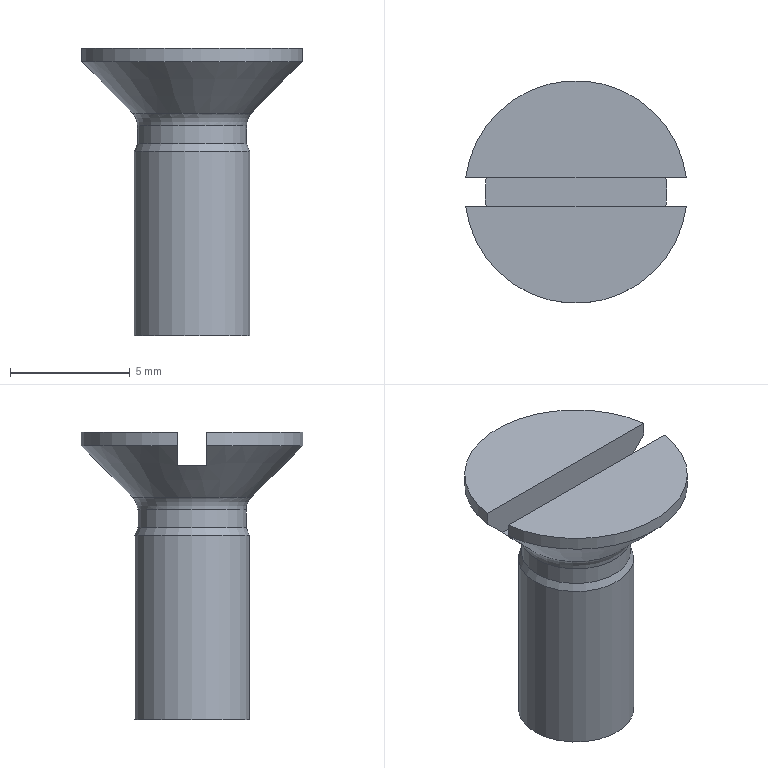Part | NX | features DATUM_CSYS 2, SKETCH 2, EXTRUDE 1, LINE 1, META 1, SWP104 1, SYMBOLIC_THREAD 1, THREADS 1 | 1 solid | 13 faces | box 9.222 x 9.3 x 12 mm | volume 279.35 mm3 | plane 6 | cylinder 4 | cone 2 | torus 1 | commonest cylinder face diameters 9.3 x2 4.555 x1 4.826 x1
STEP:
#1=CARTESIAN_POINT('',(4.611,0.6,0.));
#2=VERTEX_POINT('',#1);
#3=CARTESIAN_POINT('',(-4.611,0.6,0.));
#4=VERTEX_POINT('',#3);
#5=CARTESIAN_POINT('',(10.4,0.6,0.));
#6=DIRECTION('',(-1.,0.,0.));
#7=VECTOR('',#6,1000.);
#8=LINE('',#5,#7);
#9=EDGE_CURVE('',#2,#4,#8,.T.);
#10=ORIENTED_EDGE('',*,*,#9,.F.);
#11=CARTESIAN_POINT('',(0.,0.,0.));
#12=DIRECTION('',(0.,0.,-1.));
#13=DIRECTION('',(-1.,0.,0.));
#14=AXIS2_PLACEMENT_3D('',#11,#12,#13);
#15=CIRCLE('',#14,4.65);
#16=EDGE_CURVE('',#4,#2,#15,.T.);
#17=ORIENTED_EDGE('',*,*,#16,.F.);
#18=EDGE_LOOP('',(#10,#17));
#19=FACE_BOUND('',#18,.T.);
#20=CARTESIAN_POINT('',(0.,0.,0.));
#21=DIRECTION('',(0.,0.,-1.));
#22=DIRECTION('',(-1.,0.,0.));
#23=AXIS2_PLACEMENT_3D('',#20,#21,#22);
#24=PLANE('',#23);
#25=ADVANCED_FACE('',(#19),#24,.F.);
#26=ORIENTED_EDGE('',*,*,#16,.T.);
#27=CARTESIAN_POINT('',(4.611,0.6,-0.55));
#28=VERTEX_POINT('',#27);
#29=CARTESIAN_POINT('',(4.611,0.6,0.));
#30=DIRECTION('',(0.,0.,-1.));
#31=VECTOR('',#30,1000.);
#32=LINE('',#29,#31);
#33=EDGE_CURVE('',#2,#28,#32,.T.);
#34=ORIENTED_EDGE('',*,*,#33,.T.);
#35=CARTESIAN_POINT('',(-4.611,0.6,-0.55));
#36=VERTEX_POINT('',#35);
#37=CARTESIAN_POINT('',(0.,0.,-0.55));
#38=DIRECTION('',(0.,0.,-1.));
#39=DIRECTION('',(-1.,0.,0.));
#40=AXIS2_PLACEMENT_3D('',#37,#38,#39);
#41=CIRCLE('',#40,4.65);
#42=EDGE_CURVE('',#36,#28,#41,.T.);
#43=ORIENTED_EDGE('',*,*,#42,.F.);
#44=CARTESIAN_POINT('',(-4.611,0.6,0.));
#45=DIRECTION('',(0.,0.,-1.));
#46=VECTOR('',#45,1000.);
#47=LINE('',#44,#46);
#48=EDGE_CURVE('',#36,#4,#47,.F.);
#49=ORIENTED_EDGE('',*,*,#48,.T.);
#50=EDGE_LOOP('',(#26,#34,#43,#49));
#51=FACE_BOUND('',#50,.T.);
#52=CARTESIAN_POINT('',(0.,0.,0.));
#53=DIRECTION('',(0.,0.,-1.));
#54=DIRECTION('',(-1.,0.,0.));
#55=AXIS2_PLACEMENT_3D('',#52,#53,#54);
#56=CYLINDRICAL_SURFACE('',#55,4.65);
#57=ADVANCED_FACE('',(#51),#56,.T.);
#58=CARTESIAN_POINT('',(-2.413,0.,-4.3));
#59=VERTEX_POINT('',#58);
#60=CARTESIAN_POINT('',(0.,0.,-4.3));
#61=DIRECTION('',(0.,0.,-1.));
#62=DIRECTION('',(-1.,0.,0.));
#63=AXIS2_PLACEMENT_3D('',#60,#61,#62);
#64=CIRCLE('',#63,2.413);
#65=EDGE_CURVE('',#59,#59,#64,.T.);
#66=ORIENTED_EDGE('',*,*,#65,.F.);
#67=EDGE_LOOP('',(#66));
#68=FACE_BOUND('',#67,.T.);
#69=CARTESIAN_POINT('',(-2.277,0.,-3.98));
#70=VERTEX_POINT('',#69);
#71=CARTESIAN_POINT('',(0.,0.,-3.98));
#72=DIRECTION('',(0.,0.,-1.));
#73=DIRECTION('',(-1.,0.,0.));
#74=AXIS2_PLACEMENT_3D('',#71,#72,#73);
#75=CIRCLE('',#74,2.277);
#76=EDGE_CURVE('',#70,#70,#75,.T.);
#77=ORIENTED_EDGE('',*,*,#76,.T.);
#78=EDGE_LOOP('',(#77));
#79=FACE_BOUND('',#78,.T.);
#80=CARTESIAN_POINT('',(0.,0.,-3.98));
#81=DIRECTION('',(0.,0.,-1.));
#82=DIRECTION('',(-1.,0.,0.));
#83=AXIS2_PLACEMENT_3D('',#80,#81,#82);
#84=CONICAL_SURFACE('',#83,2.277,0.4005);
#85=ADVANCED_FACE('',(#68,#79),#84,.T.);
#86=CARTESIAN_POINT('',(-2.413,0.,-12.));
#87=VERTEX_POINT('',#86);
#88=CARTESIAN_POINT('',(0.,0.,-12.));
#89=DIRECTION('',(0.,0.,-1.));
#90=DIRECTION('',(-1.,0.,0.));
#91=AXIS2_PLACEMENT_3D('',#88,#89,#90);
#92=CIRCLE('',#91,2.413);
#93=EDGE_CURVE('',#87,#87,#92,.T.);
#94=ORIENTED_EDGE('',*,*,#93,.F.);
#95=EDGE_LOOP('',(#94));
#96=FACE_BOUND('',#95,.T.);
#97=ORIENTED_EDGE('',*,*,#65,.T.);
#98=EDGE_LOOP('',(#97));
#99=FACE_BOUND('',#98,.T.);
#100=CARTESIAN_POINT('',(0.,0.,0.));
#101=DIRECTION('',(0.,0.,-1.));
#102=DIRECTION('',(-1.,0.,0.));
#103=AXIS2_PLACEMENT_3D('',#100,#101,#102);
#104=CYLINDRICAL_SURFACE('',#103,2.413);
#105=ADVANCED_FACE('',(#96,#99),#104,.T.);
#106=ORIENTED_EDGE('',*,*,#93,.T.);
#107=EDGE_LOOP('',(#106));
#108=FACE_BOUND('',#107,.T.);
#109=CARTESIAN_POINT('',(0.,2.413,-12.));
#110=DIRECTION('',(0.,0.,1.));
#111=DIRECTION('',(1.,0.,0.));
#112=AXIS2_PLACEMENT_3D('',#109,#110,#111);
#113=PLANE('',#112);
#114=ADVANCED_FACE('',(#108),#113,.F.);
#115=CARTESIAN_POINT('',(4.611,-0.6,0.));
#116=VERTEX_POINT('',#115);
#117=CARTESIAN_POINT('',(-4.611,-0.6,0.));
#118=VERTEX_POINT('',#117);
#119=CARTESIAN_POINT('',(0.,0.,0.));
#120=DIRECTION('',(0.,0.,-1.));
#121=DIRECTION('',(-1.,0.,0.));
#122=AXIS2_PLACEMENT_3D('',#119,#120,#121);
#123=CIRCLE('',#122,4.65);
#124=EDGE_CURVE('',#116,#118,#123,.T.);
#125=ORIENTED_EDGE('',*,*,#124,.F.);
#126=CARTESIAN_POINT('',(10.4,-0.6,0.));
#127=DIRECTION('',(-1.,0.,0.));
#128=VECTOR('',#127,1000.);
#129=LINE('',#126,#128);
#130=EDGE_CURVE('',#116,#118,#129,.T.);
#131=ORIENTED_EDGE('',*,*,#130,.T.);
#132=EDGE_LOOP('',(#125,#131));
#133=FACE_BOUND('',#132,.T.);
#134=CARTESIAN_POINT('',(0.,0.,0.));
#135=DIRECTION('',(0.,0.,-1.));
#136=DIRECTION('',(-1.,0.,0.));
#137=AXIS2_PLACEMENT_3D('',#134,#135,#136);
#138=PLANE('',#137);
#139=ADVANCED_FACE('',(#133),#138,.F.);
#140=ORIENTED_EDGE('',*,*,#124,.T.);
#141=CARTESIAN_POINT('',(-4.611,-0.6,-0.55));
#142=VERTEX_POINT('',#141);
#143=CARTESIAN_POINT('',(-4.611,-0.6,0.));
#144=DIRECTION('',(0.,0.,-1.));
#145=VECTOR('',#144,1000.);
#146=LINE('',#143,#145);
#147=EDGE_CURVE('',#118,#142,#146,.T.);
#148=ORIENTED_EDGE('',*,*,#147,.T.);
#149=CARTESIAN_POINT('',(4.611,-0.6,-0.55));
#150=VERTEX_POINT('',#149);
#151=CARTESIAN_POINT('',(0.,0.,-0.55));
#152=DIRECTION('',(0.,0.,-1.));
#153=DIRECTION('',(-1.,0.,0.));
#154=AXIS2_PLACEMENT_3D('',#151,#152,#153);
#155=CIRCLE('',#154,4.65);
#156=EDGE_CURVE('',#150,#142,#155,.T.);
#157=ORIENTED_EDGE('',*,*,#156,.F.);
#158=CARTESIAN_POINT('',(4.611,-0.6,0.));
#159=DIRECTION('',(0.,0.,-1.));
#160=VECTOR('',#159,1000.);
#161=LINE('',#158,#160);
#162=EDGE_CURVE('',#150,#116,#161,.F.);
#163=ORIENTED_EDGE('',*,*,#162,.T.);
#164=EDGE_LOOP('',(#140,#148,#157,#163));
#165=FACE_BOUND('',#164,.T.);
#166=CARTESIAN_POINT('',(0.,0.,0.));
#167=DIRECTION('',(0.,0.,-1.));
#168=DIRECTION('',(-1.,0.,0.));
#169=AXIS2_PLACEMENT_3D('',#166,#167,#168);
#170=CYLINDRICAL_SURFACE('',#169,4.65);
#171=ADVANCED_FACE('',(#165),#170,.T.);
#172=CARTESIAN_POINT('',(-2.5,0.,-2.7));
#173=VERTEX_POINT('',#172);
#174=CARTESIAN_POINT('',(0.,0.,-2.7));
#175=DIRECTION('',(0.,0.,-1.));
#176=DIRECTION('',(-1.,0.,0.));
#177=AXIS2_PLACEMENT_3D('',#174,#175,#176);
#178=CIRCLE('',#177,2.5);
#179=EDGE_CURVE('',#173,#173,#178,.T.);
#180=ORIENTED_EDGE('',*,*,#179,.F.);
#181=EDGE_LOOP('',(#180));
#182=FACE_BOUND('',#181,.T.);
#183=CARTESIAN_POINT('',(-3.752,-0.6,-1.4));
#184=VERTEX_POINT('',#183);
#185=CARTESIAN_POINT('',(-3.752,0.6,-1.4));
#186=VERTEX_POINT('',#185);
#187=CARTESIAN_POINT('',(0.,0.,-1.4));
#188=DIRECTION('',(0.,0.,-1.));
#189=DIRECTION('',(-1.,0.,0.));
#190=AXIS2_PLACEMENT_3D('',#187,#188,#189);
#191=CIRCLE('',#190,3.8);
#192=EDGE_CURVE('',#184,#186,#191,.T.);
#193=ORIENTED_EDGE('',*,*,#192,.T.);
#194=CARTESIAN_POINT('',(-3.752,0.6,-1.4));
#195=CARTESIAN_POINT('',(-4.039,0.6,-1.117));
#196=CARTESIAN_POINT('',(-4.325,0.6,-0.8336));
#197=CARTESIAN_POINT('',(-4.611,0.6,-0.55));
#198=B_SPLINE_CURVE_WITH_KNOTS('',3,(#194,#195,#196,#197),.UNSPECIFIED.,.F.,.F.,(4,4),(0.01911,0.02032),.UNSPECIFIED.);
#199=EDGE_CURVE('',#186,#36,#198,.T.);
#200=ORIENTED_EDGE('',*,*,#199,.T.);
#201=ORIENTED_EDGE('',*,*,#42,.T.);
#202=CARTESIAN_POINT('',(3.752,0.6,-1.4));
#203=VERTEX_POINT('',#202);
#204=CARTESIAN_POINT('',(4.611,0.6,-0.55));
#205=CARTESIAN_POINT('',(4.325,0.6,-0.8336));
#206=CARTESIAN_POINT('',(4.039,0.6,-1.117));
#207=CARTESIAN_POINT('',(3.752,0.6,-1.4));
#208=B_SPLINE_CURVE_WITH_KNOTS('',3,(#204,#205,#206,#207),.UNSPECIFIED.,.F.,.F.,(4,4),(0.00794,0.009148),.UNSPECIFIED.);
#209=EDGE_CURVE('',#28,#203,#208,.T.);
#210=ORIENTED_EDGE('',*,*,#209,.T.);
#211=CARTESIAN_POINT('',(3.752,-0.6,-1.4));
#212=VERTEX_POINT('',#211);
#213=CARTESIAN_POINT('',(0.,0.,-1.4));
#214=DIRECTION('',(0.,0.,-1.));
#215=DIRECTION('',(-1.,0.,0.));
#216=AXIS2_PLACEMENT_3D('',#213,#214,#215);
#217=CIRCLE('',#216,3.8);
#218=EDGE_CURVE('',#203,#212,#217,.T.);
#219=ORIENTED_EDGE('',*,*,#218,.T.);
#220=CARTESIAN_POINT('',(3.752,-0.6,-1.4));
#221=CARTESIAN_POINT('',(4.039,-0.6,-1.117));
#222=CARTESIAN_POINT('',(4.325,-0.6,-0.8336));
#223=CARTESIAN_POINT('',(4.611,-0.6,-0.55));
#224=B_SPLINE_CURVE_WITH_KNOTS('',3,(#220,#221,#222,#223),.UNSPECIFIED.,.F.,.F.,(4,4),(0.01911,0.02032),.UNSPECIFIED.);
#225=EDGE_CURVE('',#212,#150,#224,.T.);
#226=ORIENTED_EDGE('',*,*,#225,.T.);
#227=ORIENTED_EDGE('',*,*,#156,.T.);
#228=CARTESIAN_POINT('',(-4.611,-0.6,-0.55));
#229=CARTESIAN_POINT('',(-4.325,-0.6,-0.8336));
#230=CARTESIAN_POINT('',(-4.039,-0.6,-1.117));
#231=CARTESIAN_POINT('',(-3.752,-0.6,-1.4));
#232=B_SPLINE_CURVE_WITH_KNOTS('',3,(#228,#229,#230,#231),.UNSPECIFIED.,.F.,.F.,(4,4),(0.00794,0.009148),.UNSPECIFIED.);
#233=EDGE_CURVE('',#142,#184,#232,.T.);
#234=ORIENTED_EDGE('',*,*,#233,.T.);
#235=EDGE_LOOP('',(#193,#200,#201,#210,#219,#226,#227,#234));
#236=FACE_BOUND('',#235,.T.);
#237=CARTESIAN_POINT('',(0.,0.,-0.55));
#238=DIRECTION('',(0.,0.,1.));
#239=DIRECTION('',(1.,0.,0.));
#240=AXIS2_PLACEMENT_3D('',#237,#238,#239);
#241=CONICAL_SURFACE('',#240,4.65,0.7854);
#242=ADVANCED_FACE('',(#182,#236),#241,.T.);
#243=CARTESIAN_POINT('',(-2.277,0.,-3.237));
#244=VERTEX_POINT('',#243);
#245=CARTESIAN_POINT('',(0.,0.,-3.237));
#246=DIRECTION('',(0.,0.,-1.));
#247=DIRECTION('',(-1.,0.,0.));
#248=AXIS2_PLACEMENT_3D('',#245,#246,#247);
#249=CIRCLE('',#248,2.277);
#250=EDGE_CURVE('',#244,#244,#249,.T.);
#251=ORIENTED_EDGE('',*,*,#250,.F.);
#252=EDGE_LOOP('',(#251));
#253=FACE_BOUND('',#252,.T.);
#254=ORIENTED_EDGE('',*,*,#179,.T.);
#255=EDGE_LOOP('',(#254));
#256=FACE_BOUND('',#255,.T.);
#257=CARTESIAN_POINT('',(0.,0.,-3.237));
#258=DIRECTION('',(0.,0.,-1.));
#259=DIRECTION('',(-1.,0.,0.));
#260=AXIS2_PLACEMENT_3D('',#257,#258,#259);
#261=TOROIDAL_SURFACE('',#260,3.037,0.7597);
#262=ADVANCED_FACE('',(#253,#256),#261,.F.);
#263=ORIENTED_EDGE('',*,*,#76,.F.);
#264=EDGE_LOOP('',(#263));
#265=FACE_BOUND('',#264,.T.);
#266=ORIENTED_EDGE('',*,*,#250,.T.);
#267=EDGE_LOOP('',(#266));
#268=FACE_BOUND('',#267,.T.);
#269=CARTESIAN_POINT('',(0.,0.,0.));
#270=DIRECTION('',(0.,0.,-1.));
#271=DIRECTION('',(-1.,0.,0.));
#272=AXIS2_PLACEMENT_3D('',#269,#270,#271);
#273=CYLINDRICAL_SURFACE('',#272,2.277);
#274=ADVANCED_FACE('',(#265,#268),#273,.T.);
#275=ORIENTED_EDGE('',*,*,#9,.T.);
#276=ORIENTED_EDGE('',*,*,#48,.F.);
#277=ORIENTED_EDGE('',*,*,#199,.F.);
#278=CARTESIAN_POINT('',(10.4,0.6,-1.4));
#279=DIRECTION('',(-1.,0.,0.));
#280=VECTOR('',#279,1000.);
#281=LINE('',#278,#280);
#282=EDGE_CURVE('',#203,#186,#281,.T.);
#283=ORIENTED_EDGE('',*,*,#282,.F.);
#284=ORIENTED_EDGE('',*,*,#209,.F.);
#285=ORIENTED_EDGE('',*,*,#33,.F.);
#286=EDGE_LOOP('',(#275,#276,#277,#283,#284,#285));
#287=FACE_BOUND('',#286,.T.);
#288=CARTESIAN_POINT('',(10.4,0.6,0.));
#289=DIRECTION('',(0.,1.,0.));
#290=DIRECTION('',(0.,0.,1.));
#291=AXIS2_PLACEMENT_3D('',#288,#289,#290);
#292=PLANE('',#291);
#293=ADVANCED_FACE('',(#287),#292,.F.);
#294=ORIENTED_EDGE('',*,*,#282,.T.);
#295=ORIENTED_EDGE('',*,*,#192,.F.);
#296=CARTESIAN_POINT('',(10.4,-0.6,-1.4));
#297=DIRECTION('',(-1.,0.,0.));
#298=VECTOR('',#297,1000.);
#299=LINE('',#296,#298);
#300=EDGE_CURVE('',#212,#184,#299,.T.);
#301=ORIENTED_EDGE('',*,*,#300,.F.);
#302=ORIENTED_EDGE('',*,*,#218,.F.);
#303=EDGE_LOOP('',(#294,#295,#301,#302));
#304=FACE_BOUND('',#303,.T.);
#305=CARTESIAN_POINT('',(10.4,0.,-1.4));
#306=DIRECTION('',(0.,0.,-1.));
#307=DIRECTION('',(-1.,0.,0.));
#308=AXIS2_PLACEMENT_3D('',#305,#306,#307);
#309=PLANE('',#308);
#310=ADVANCED_FACE('',(#304),#309,.F.);
#311=ORIENTED_EDGE('',*,*,#130,.F.);
#312=ORIENTED_EDGE('',*,*,#162,.F.);
#313=ORIENTED_EDGE('',*,*,#225,.F.);
#314=ORIENTED_EDGE('',*,*,#300,.T.);
#315=ORIENTED_EDGE('',*,*,#233,.F.);
#316=ORIENTED_EDGE('',*,*,#147,.F.);
#317=EDGE_LOOP('',(#311,#312,#313,#314,#315,#316));
#318=FACE_BOUND('',#317,.T.);
#319=CARTESIAN_POINT('',(10.4,-0.6,-1.4));
#320=DIRECTION('',(0.,-1.,0.));
#321=DIRECTION('',(0.,0.,-1.));
#322=AXIS2_PLACEMENT_3D('',#319,#320,#321);
#323=PLANE('',#322);
#324=ADVANCED_FACE('',(#318),#323,.F.);
#325=CLOSED_SHELL('',(#25,#57,#85,#105,#114,#139,#171,#242,#262,#274,#293,#310,#324));
#326=MANIFOLD_SOLID_BREP('',#325);
#327=(LENGTH_UNIT()NAMED_UNIT(*)SI_UNIT(.MILLI.,.METRE.));
#328=UNCERTAINTY_MEASURE_WITH_UNIT(LENGTH_MEASURE(0.0508),#327,'','');
#329=(NAMED_UNIT(*)PLANE_ANGLE_UNIT()SI_UNIT($,.RADIAN.));
#330=(NAMED_UNIT(*)SI_UNIT($,.STERADIAN.)SOLID_ANGLE_UNIT());
#331=(GEOMETRIC_REPRESENTATION_CONTEXT(3)GLOBAL_UNCERTAINTY_ASSIGNED_CONTEXT((#328))GLOBAL_UNIT_ASSIGNED_CONTEXT((#327,#329,#330))REPRESENTATION_CONTEXT('',''));
#332=ADVANCED_BREP_SHAPE_REPRESENTATION('',(#326),#331);